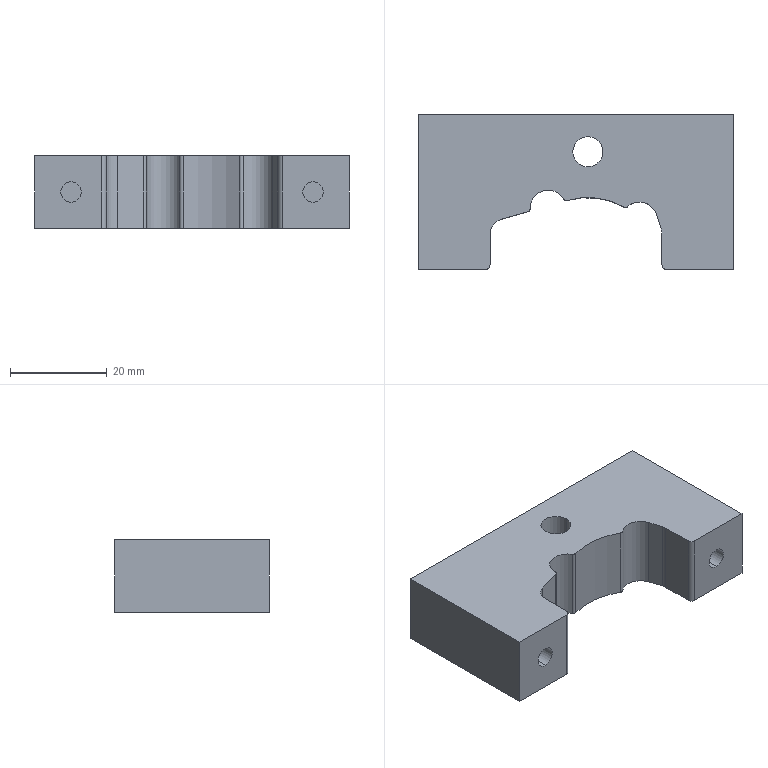NC program | Mastercam | posted with a generic post
Lines 25 to 726 of 2481:
N230 T9 M6
N240 G0 G90 G17 G54 X-45.614 Y-30.265 A0. S6000 M3
N250 G43 H9 Z50.
N260 Z2.
N270 G1 Z-15.75 F2000.
N280 X-45.889 Y-29.487 Z-15.877 F4000.
N290 G3 X-46.313 Y-28.813 Z-16. I-1.697 J-.599
N300 G2 X-47.51 Y-26.707 I5.557 J4.549
N310 X-47.895 Y-24.67 I7.524 J2.477
N320 X-47.955 Y-22.296 I47.214 J2.374
N330 X-47.943 Y-21.288 I47.274 J0.
N340 X-47.932 Y-20.029 I986.819 J-8.394
N350 G1 X-47.929 Y-19.714
N360 X-47.612 Y11.998
N370 X-47.499 Y22.913
N380 G2 X-47.09 Y25.288 I7.557 J-.078
N390 X-44.537 Y28.308 I5.258 J-1.857
N400 X-41.791 Y29.334 I4.597 J-8.114
N410 X-38.089 Y29.777 I4.617 J-22.923
N420 X-32.309 Y29.894 I5.78 J-143.246
N430 X-31.772 Y29.892 I0. J-143.363
N440 X-29.817 Y29.897 I3.277 J-998.552
N450 G1 X-29.492
N460 X2.98 Y29.9
N470 X35.449
N480 G2 X36.585 Y29.901 I1.136 J-880.668
N490 X40.411 Y29.892 I0. J-880.669
N500 X43.057 Y29.37 I-.083 J-7.387
N510 X45.814 Y26.904 I-2.177 J-5.207
N520 X46.836 Y24.158 I-8.139 J-4.595
N530 X47.277 Y20.458 I-22.99 J-4.615
N540 X47.393 Y14.679 I-143.703 J-5.779
N550 X47.392 Y14.141 I-143.819 J0.
N560 X47.396 Y12.512 I-914.774 J-3.05
N570 G1 X47.397 Y12.187
N580 X47.4 Y-20.286
N590 G2 X47.401 Y-20.936 I-181.849 J-.65
N600 X47.39 Y-22.995 I-181.85 J0.
N610 X46.829 Y-25.653 I-7.232 J.136
N620 X44.318 Y-28.363 I-5.202 J2.303
N630 X41.384 Y-29.394 I-4.683 J8.636
N640 X37.72 Y-29.789 I-4.561 J25.118
N650 X31.559 Y-29.897 I-6.161 J176.47
N660 X30.765 Y-29.895 I0. J176.578
N670 G1 X30.439
N680 X-2.036 Y-29.9
N690 X-34.504
N700 X-40.449 Y-29.891
N710 G2 X-42.643 Y-29.509 I.097 J7.049
N720 X-45.36 Y-27.368 I1.999 J5.331
N730 X-46.578 Y-24.594 I7.011 J4.733
N740 X-47.068 Y-21.166 I18.144 J4.342
N750 X-47.178 Y-16.743 I88.951 J4.423
N760 X-47.173 Y-15.771 I89.061 J0.
N770 X-47.13 Y-9.905 I968.214 J-4.162
N780 G1 X-47.127 Y-9.581
N790 X-46.811 Y21.335
N800 G2 X-46.545 Y23.383 I8.429 J-.053
N810 X-44.207 Y26.771 I6.177 J-1.762
N820 X-41.382 Y28.209 I5.544 J-7.399
N830 X-37.947 Y28.896 I5.105 J-16.599
N840 X-32.805 Y29.157 I5.493 J-57.43
N850 X-23.221 Y29.203 I9.584 J-998.899
N860 X-20.74 Y29.2 I0. J-998.945
N870 G1 X-20.415
N880 X12.054
N890 X38.75 Y29.191
N900 X38.76
N910 G2 X40.794 Y28.949 I0. J-8.644
N920 X44.217 Y26.656 I-1.659 J-6.178
N930 X45.685 Y23.834 I-7.243 J-5.561
N940 X46.388 Y20.391 I-16.3 J-5.124
N950 X46.65 Y15.576 I-54.549 J-5.373
N960 X46.704 Y5.699 I-910.196 J-9.877
N970 X46.7 Y3.178 I-910.25 J0.
N980 G1 Y2.853
N990 X46.691 Y-21.246
N1000 Y-21.257
N1010 G2 X46.451 Y-23.287 I-8.672 J0.
N1020 X44.161 Y-26.713 I-6.178 J1.651
N1030 X41.339 Y-28.183 I-5.562 J7.231
N1040 X37.896 Y-28.888 I-5.124 J16.276
N1050 X33.08 Y-29.149 I-5.375 J54.481
N1060 X23.203 Y-29.203 I-9.877 J908.925
N1070 X20.681 Y-29.2 I0. J908.979
N1080 G1 X20.357
N1090 X-12.112
N1100 X-38.82 Y-29.19
N1110 X-38.83
N1120 G2 X-41.221 Y-28.777 I0. J7.137
N1130 X-44.103 Y-26.61 I2.341 J6.114
N1140 X-45.546 Y-23.777 I7.31 J5.507
N1150 X-46.22 Y-20.326 I16.303 J4.976
N1160 X-46.436 Y-15.507 I54.432 J4.852
N1170 G1 Y-14.598
N1180 G2 X-46.363 Y-3.108 I897.862 J0.
N1190 G1 X-46.36 Y-2.783
N1200 X-46.129 Y19.67
N1210 G2 X-45.821 Y22.09 I9.687 J-.004
N1220 X-43.504 Y25.623 I6.853 J-1.968
N1230 X-40.379 Y27.338 I6.19 J-7.578
N1240 X-36.6 Y28.145 I5.691 J-17.4
N1250 X-31.451 Y28.441 I5.758 J-55.184
N1260 X-21.727 Y28.503 I9.724 J-760.399
N1270 X-19.373 Y28.499 I0. J-760.461
N1280 G1 X-19.048
N1290 X13.422 Y28.5
N1300 X37.185 Y28.492
N1310 X37.233
N1320 G2 X39.63 Y28.181 I0. J-9.402
N1330 X43.151 Y25.845 I-2. J-6.838
N1340 X44.851 Y22.717 I-7.645 J-6.179
N1350 X45.649 Y18.941 I-17.546 J-5.681
N1360 X45.942 Y13.795 I-55.737 J-5.753
N1370 X46.003 Y4.073 I-769.313 J-9.722
N1380 X45.999 Y1.717 I-769.374 J0.
N1390 G1 Y1.392
N1400 X45.989 Y-19.784
N1410 Y-19.791
N1420 G2 X45.642 Y-22.262 I-8.962 J0.
N1430 X43.244 Y-25.734 I-6.83 J2.153
N1440 X40.109 Y-27.387 I-6.151 J7.865
N1450 X36.343 Y-28.16 I-5.655 J17.992
N1460 X31.204 Y-28.443 I-5.741 J57.339
N1470 X21.208 Y-28.502 I-9.996 J840.155
N1480 X18.804 Y-28.499 I0. J840.214
N1490 G1 X18.479 Y-28.5
N1500 X-13.99
N1510 X-37.099 Y-28.493
N1520 X-37.145
N1530 G2 X-39.581 Y-28.156 I0. J8.963
N1540 X-43.064 Y-25.764 I2.114 J6.813
N1550 X-44.718 Y-22.618 I7.782 J6.097
N1560 X-45.471 Y-18.838 I17.743 J5.502
N1570 X-45.711 Y-13.691 I56.177 J5.193
N1580 X-45.714 Y-11.688 I772.695 J2.003
N1590 X-45.648 Y-1.614 I772.698 J0.
N1600 G1 X-45.644 Y-1.289
N1610 X-45.442 Y18.245
N1620 G2 X-45.128 Y20.796 I11.216 J-.086
N1630 X-42.518 Y24.805 I7.408 J-1.969
N1640 X-39.448 Y26.501 I6.467 J-8.078
N1650 X-35.684 Y27.368 I5.973 J-17.338
N1660 X-30.512 Y27.719 I6.026 J-50.413
N1670 X-21.626 Y27.8 I8.886 J-485.482
N1680 X-20.04 Y27.798 I0. J-485.563
N1690 G1 X-19.715
N1700 X12.755 Y27.8
N1710 X35.887 Y27.787
N1720 G2 X38.491 Y27.435 I-.066 J-10.297
N1730 X42.438 Y24.72 I-2.176 J-7.39
N1740 X44.193 Y21.249 I-8.694 J-6.574
N1750 X44.972 Y17.172 I-20.126 J-5.957
N1760 X45.246 Y11.73 I-67.431 J-6.124
N1770 X45.304 Y1.065 I-987.723 J-10.665
N1780 X45.3 Y-1.639 I-987.781 J0.
N1790 G1 Y-1.964
N1800 X45.29 Y-18.262
N1810 G2 X44.979 Y-20.833 I-10.873 J.011
N1820 X42.343 Y-24.84 I-7.391 J1.991
N1830 X39.269 Y-26.519 I-6.448 J8.154
N1840 X35.509 Y-27.374 I-5.959 J17.514
N1850 X30.34 Y-27.721 I-6.019 J51.043
N1860 X21.457 Y-27.801 I-8.883 J492.934
N1870 X19.87 Y-27.798 I0. J493.014
N1880 G1 X19.545
N1890 X-12.926 Y-27.8
N1900 X-35.728 Y-27.789
N1910 G2 X-38.335 Y-27.439 I.05 J10.265
N1920 X-42.147 Y-24.884 I2.152 J7.333
N1930 X-43.834 Y-21.799 I8.025 J6.392
N1940 X-44.674 Y-18.024 I17.221 J5.811
N1950 X-44.979 Y-12.845 I49.968 J5.537
N1960 X-44.997 Y-8.745 I478.968 J4.1
N1970 X-44.954 Y-2.372 I478.986 J0.
N1980 G1 X-44.951 Y-2.047
N1990 X-44.755 Y16.84
N2000 G2 X-44.504 Y19.282 I13.738 J-.174
N2010 X-41.214 Y24.29 I8.022 J-1.687
N2020 X-37.776 Y25.953 I6.71 J-9.482
N2030 X-33.725 Y26.736 I6.138 J-20.895
N2040 X-27.946 Y27.041 I6.433 J-67.056
N2050 X-17.339 Y27.103 I10.607 J-910.669
N2060 X-14.9 Y27.099 I0. J-910.731
N2070 G1 X-14.575
N2080 X17.894 Y27.1
N2090 X34.174 Y27.092
N2100 X34.184
N2110 G2 X36.588 Y26.893 I0. J-14.562
N2120 X41.682 Y23.722 I-1.447 J-8.003
N2130 X43.407 Y20.291 I-9.216 J-6.782
N2140 X44.221 Y16.227 I-20.23 J-6.168
N2150 X44.531 Y10.771 I-63.111 J-6.321
N2160 X44.602 Y.838 I-696.262 J-9.933
N2170 X44.599 Y-1.31 I-696.333 J0.
N2180 G1 Y-1.635
N2190 X44.587 Y-16.97
N2200 G2 X44.315 Y-19.461 I-12.601 J.113
N2210 X41.285 Y-24.134 I-7.919 J1.816
N2220 X37.858 Y-25.885 I-6.8 J9.079
N2230 X33.789 Y-26.715 I-6.184 J19.95
N2240 X28.328 Y-27.03 I-6.329 J62.114
N2250 X18.54 Y-27.102 I-9.788 J669.314
N2260 X16.571 Y-27.099 I0. J669.386
N2270 G1 X16.246
N2280 X-16.223 Y-27.1
N2290 X-34.135 Y-27.091
N2300 G2 X-36.581 Y-26.866 I.023 J13.644
N2310 X-41.338 Y-23.95 I1.566 J7.893
N2320 X-43.148 Y-20.518 I8.686 J6.774
N2330 X-43.986 Y-16.424 I19.104 J6.044
N2340 X-44.267 Y-10.947 I58.989 J5.766
N2350 X-44.278 Y-7.384 I596.981 J3.563
N2360 X-44.226 Y.49 I596.992 J0.
N2370 G1 X-44.223 Y.815
N2380 X-44.067 Y15.479
N2390 G2 X-43.781 Y18.264 I15.659 J-.203
N2400 X-40.26 Y23.544 I8.409 J-1.794
N2410 X-36.853 Y25.184 I6.889 J-9.948
N2420 X-32.459 Y26.032 I6.53 J-22.026
N2430 X-26.692 Y26.336 I6.554 J-69.681
N2440 X-15.997 Y26.403 I10.695 J-855.879
N2450 X-13.643 Y26.399 I0. J-855.946
N2460 G1 X-13.318
N2470 X19.151 Y26.4
N2480 X32.834 Y26.391
N2490 G2 X35.599 Y26.155 I-.008 J-16.392
N2500 X40.957 Y22.737 I-1.575 J-8.378
N2510 X42.646 Y19.334 I-9.716 J-6.944
N2520 X43.481 Y15.285 I-20.512 J-6.338
N2530 X43.818 Y9.82 I-60.646 J-6.486
N2540 X43.9 Y.335 I-548.288 J-9.485
N2550 X43.898 Y-1.295 I-548.37 J0.
N2560 G1 Y-1.62
N2570 X43.892 Y-15.303
N2580 Y-15.311
N2590 G2 X43.663 Y-18.059 I-16.613 J0.
N2600 X40.27 Y-23.433 I-8.379 J1.532
N2610 X36.869 Y-25.135 I-6.954 J9.645
N2620 X32.817 Y-25.977 I-6.346 J20.37
N2630 X27.351 Y-26.317 I-6.49 J60.165
N2640 X17.864 Y-26.4 I-9.487 J543.312
N2650 X16.235 Y-26.398 I0. J543.395
N2660 G1 X15.91
N2670 X-16.561 Y-26.4
N2680 X-32.853 Y-26.389
N2690 G2 X-35.664 Y-26.111 I.061 J14.961
N2700 X-40.665 Y-22.896 I1.77 J8.248
N2710 X-42.403 Y-19.486 I9.334 J6.908
N2720 X-43.243 Y-15.413 I19.709 J6.188
N2730 X-43.545 Y-9.932 I58.101 J5.944
N2740 X-43.564 Y-5.625 I492.643 J4.307
N2750 X-43.521 Y.862 I492.662 J0.
N2760 G1 X-43.518 Y1.187
N2770 X-43.378 Y14.231
N2780 G2 X-43.132 Y16.942 I18.18 J-.284
N2790 X-39.225 Y22.882 I8.819 J-1.545
N2800 X-35.461 Y24.574 I7.187 J-10.954
N2810 X-31.112 Y25.345 I6.578 J-24.472
N2820 X-25.031 Y25.64 I6.879 J-78.864
N2830 X-14.126 Y25.702 I10.905 J-956.982
N2840 X-11.664 Y25.699 I0. J-957.044
N2850 G1 X-11.339
N2860 X21.13 Y25.7
N2870 X31.567 Y25.69
N2880 G2 X34.256 Y25.494 I-.058 J-19.277
N2890 X40.287 Y21.715 I-1.302 J-8.781
N2900 X42.035 Y17.954 I-10.584 J-7.206
N2910 X42.833 Y13.594 I-23.775 J-6.601
N2920 X43.138 Y7.507 I-76.485 J-6.888
N2930 X43.202 Y-3.674 I-972.393 J-11.181
N2940 X43.199 Y-6.187 I-972.457 J0.
N2950 G1 Y-6.512
N2960 G2 X43.201 Y-8.586 I-990.829 J-2.074
N2970 X43.185 Y-14.374 I-990.831 J0.
N2980 X42.926 Y-17.13 I-16.565 J.166
N2990 X39.259 Y-22.756 I-8.703 J1.664
N3000 X35.5 Y-24.522 I-7.226 J10.499
N3010 X31.137 Y-25.328 I-6.61 J23.555
N3020 X25.048 Y-25.637 I-6.893 J75.679
N3030 X13.866 Y-25.702 I-11.182 J960.7
N3040 X11.353 Y-25.699 I0. J960.765
N3050 G1 X11.028
N3060 X-21.441 Y-25.7
N3070 X-31.562 Y-25.688
N3080 G2 X-34.288 Y-25.462 I.1 J17.724
N3090 X-39.982 Y-21.887 I1.465 J8.657
N3100 X-41.782 Y-18.117 I10.155 J7.164
N3110 X-42.581 Y-13.733 I22.793 J6.417
N3120 X-42.843 Y-7.631 I72.86 J6.183
N3130 X-42.846 Y-5.471 I876.429 J2.16
N3140 X-42.774 Y5.742 I876.432 J0.
N3150 G1 X-42.771 Y6.066
N3160 G2 X-42.681 Y13.282 I705.047 J-5.15
N3170 X-42.33 Y16.407 I16.546 J-.274
N3180 X-38.628 Y21.941 I8.971 J-1.996
N3190 X-34.898 Y23.732 I7.395 J-10.62
N3200 X-30.536 Y24.583 I6.779 J-23.139
N3210 X-24.432 Y24.925 I7.042 J-71.036
N3220 X-13.845 Y25.001 I10.587 J-735.463
N3230 X-11.704 Y24.999 I0. J-735.539
N3240 G1 X-11.379
N3250 X21.091 Y25.
N3260 X30.566 Y24.986
N3270 G2 X33.661 Y24.706 I-.041 J-17.712
N3280 X39.562 Y20.801 I-1.714 J-9.003
N3290 X41.29 Y17.061 I-10.97 J-7.335
N3300 X42.104 Y12.71 I-23.95 J-6.732
N3310 X42.429 Y6.617 I-74.089 J-7.016
N3320 X42.501 Y-4.23 I-811.991 J-10.847
N3330 X42.499 Y-6.433 I-812.063 J0.
N3340 G1 Y-6.758
N3350 G2 X42.502 Y-8.488 I-526.727 J-1.73
N3360 X42.479 Y-13.332 I-526.73 J0.
N3370 X42.136 Y-16.485 I-15.85 J.133
N3380 X38.389 Y-22.001 I-8.915 J2.024
N3390 X34.652 Y-23.762 I-7.36 J10.771
N3400 X30.295 Y-24.594 I-6.751 J23.53
N3410 X24.197 Y-24.928 I-7.026 J72.615
N3420 X13.615 Y-25.002 I-10.582 J756.421
N3430 X11.47 Y-24.999 I0. J756.495
N3440 G1 X11.145
N3450 X-21.325 Y-25.
N3460 X-30.479 Y-24.985
N3470 G2 X-33.594 Y-24.687 I.054 J17.024
N3480 X-39.196 Y-21.051 I1.778 J8.874
N3490 X-41.004 Y-17.304 I10.349 J7.301
N3500 X-41.835 Y-12.924 I22.641 J6.564
N3510 X-42.119 Y-7.143 I66.163 J6.156
N3520 X-42.133 Y-3.086 I599.653 J4.057
N3530 X-42.084 Y4.619 I599.667 J0.
N3540 G1 X-42.08 Y4.944
N3550 G2 X-41.99 Y12.161 I621.71 J-4.194
N3560 X-41.673 Y15.233 I18.347 J-.343
N3570 X-37.509 Y21.381 I9.315 J-1.824
N3580 X-33.786 Y23.065 I7.439 J-11.487
N3590 X-29.097 Y23.918 I6.968 J-24.988
N3600 X-22.691 Y24.235 I7.213 J-80.934
N3610 X-11.23 Y24.302 I11.461 J-975.753
N3620 X-8.673 Y24.299 I0. J-975.82
N3630 G1 X-8.348
N3640 X24.122 Y24.3
N3650 G2 X25.391 Y24.302 I1.269 J-380.369
N3660 X29.721 Y24.277 I0. J-380.371
N3670 X32.818 Y23.968 I-.185 J-17.515
N3680 X38.703 Y20.109 I-1.828 J-9.204
N3690 X40.486 Y16.395 I-10.852 J-7.497
N3700 X41.355 Y12.039 I-23.201 J-6.892
N3710 X41.716 Y5.929 I-69.104 J-7.154
N3720 X41.8 Y-4.332 I-627.054 J-10.261
N3730 X41.798 Y-6.155 I-627.138 J0.
N3740 G1 Y-6.48
N3750 G2 X41.802 Y-8.038 I-314.958 J-1.558
N3760 X41.771 Y-12.422 I-314.962 J0.
N3770 X41.415 Y-15.559 I-16.236 J.257
N3780 X37.761 Y-21.093 I-9.121 J2.049
N3790 X34.056 Y-22.935 I-7.54 J10.515
N3800 X29.691 Y-23.837 I-6.926 J22.506
N3810 X23.904 Y-24.204 I-6.946 J63.669
N3820 X14.024 Y-24.299 I-9.88 J514.383
N3830 X12.46 Y-24.297 I0. J514.478
N3840 G1 X12.135
N3850 X-20.336 Y-24.3
N3860 X-29.155 Y-24.287
N3870 G2 X-32.176 Y-24.059 I.047 J20.752
N3880 X-36.303 Y-22.371 I1.452 J9.444
N3890 X-39.176 Y-19.029 I5.927 J8.002
N3900 X-40.651 Y-14.907 I13.556 J7.173
N3910 X-41.272 Y-9.945 I32.534 J6.594
N3920 X-41.429 Y-3.57 I129.288 J6.375
N3930 X-41.426 Y-2.62 I129.445 J0.
N3940 X-41.377 Y5.199 I994.994 J-2.291
N3950 G1 X-41.374 Y5.524
N3960 G2 X-41.283 Y11.474 I270.041 J-1.139
N3970 X-40.908 Y14.575 I17.298 J-.518
N3980 X-36.68 Y20.637 I9.481 J-2.108
N3990 X-32.973 Y22.318 I7.546 J-11.708
N4000 X-28.289 Y23.191 I7.08 J-24.98
N4010 X-21.876 Y23.527 I7.321 J-78.423
N4020 X-10.755 Y23.601 I11.121 J-831.422
N4030 X-8.503 Y23.599 I0. J-831.496
N4040 G1 X-8.178
N4050 X24.292 Y23.6
N4060 G2 X25.319 Y23.603 I1.027 J-156.116
N4070 X29.299 Y23.553 I0. J-156.119
N4080 X32.47 Y23.118 I-.468 J-15.204
N4090 X37.894 Y19.365 I-2.404 J-9.27
N4100 X39.707 Y15.674 I-10.863 J-7.626
N4110 X40.615 Y11.317 I-22.815 J-7.025
N4120 X41.005 Y5.196 I-65.895 J-7.274
N4130 X41.099 Y-5.006 I-551.649 J-10.202
N4140 X41.097 Y-6.57 I-551.743 J0.
N4150 G1 Y-6.895
N4160 G2 X41.101 Y-7.996 I-162.501 J-1.101
N4170 X41.062 Y-11.556 I-162.505 J0.
N4180 X40.689 Y-14.684 I-16.474 J.377
N4190 X36.75 Y-20.476 I-9.363 J2.133
N4200 X33.052 Y-22.246 I-7.596 J11.121
N4210 X28.352 Y-23.169 I-7.12 J23.832
N4220 X22.257 Y-23.516 I-7.219 J73.081
N4230 X11.67 Y-23.601 I-10.587 J663.08
N4240 X9.849 Y-23.598 I0. J663.165
N4250 G1 X9.525
N4260 X-22.946 Y-23.6
N4270 G2 X-24.197 Y-23.602 I-1.251 J336.019
N4280 X-28.55 Y-23.574 I0. J336.021
N4290 X-31.622 Y-23.275 I.246 J18.462
N4300 X-37.812 Y-19.193 I1.742 J9.373
N4310 X-39.541 Y-15.473 I11.187 J7.465
N4320 X-40.412 Y-10.765 I23.978 J6.868
N4330 X-40.695 Y-4.669 I73.642 J6.476
N4340 X-40.706 Y-.985 I603. J3.684
N4350 X-40.605 Y10.089 I603.011 J0.
N4360 X-40.323 Y13.094 I21.279 J-.481
N4370 X-38.701 Y17.151 I10.151 J-1.707
N4380 X-35.134 Y20.34 I8.494 J-5.91
N4390 X-31.059 Y21.875 I7.545 J-13.855
N4400 X-26.103 Y22.595 I7.162 J-31.88
N4410 X-19.092 Y22.853 I7.641 J-111.963
N4420 X-9.723 Y22.898 I9.369 J-980.312
N4430 G1 X-8.664 Y22.897
N4440 X-8.34 Y22.898
N4450 X24.132 Y22.9
N4460 G2 X24.879 Y22.903 I.747 J-103.905
N4470 X28.511 Y22.839 I0. J-103.908
N4480 X31.679 Y22.376 I-.596 J-15.166
N4490 X37.082 Y18.644 I-2.518 J-9.423
N4500 X38.928 Y14.973 I-10.786 J-7.723
N4510 X39.874 Y10.617 I-22.418 J-7.148
N4520 X40.283 Y4.818 I-60.555 J-7.182
N4530 X40.396 Y-4.825 I-409.971 J-9.643
N4540 X40.394 Y-5.989 I-410.084 J0.
N4550 G1 X40.395 Y-6.314
N4560 G2 X40.4 Y-7.353 I-106.992 J-1.039
N4570 X40.337 Y-11.024 I-106.997 J0.
N4580 X39.872 Y-14.192 I-15.098 J.596
N4590 X36.132 Y-19.591 I-9.423 J2.533
N4600 X32.46 Y-21.433 I-7.747 J10.866
N4610 X27.753 Y-22.419 I-7.265 J22.935
N4620 X21.642 Y-22.802 I-7.344 J68.221
N4630 X11.373 Y-22.898 I-10.269 J547.19
N4640 X9.875 Y-22.897 I0. J547.286
N4650 G1 X9.55
N4660 X-22.921 Y-22.9
N4670 G2 X-23.925 Y-22.903 I-1.004 J182.05
N4680 X-27.908 Y-22.859 I0. J182.053
N4690 X-31.012 Y-22.499 I.43 J17.255
N4700 X-37.101 Y-18.317 I2.053 J9.514
N4710 X-38.808 Y-14.609 I11.499 J7.54
N4720 X-39.684 Y-9.909 I24.253 J6.953
N4730 X-39.979 Y-3.811 I72.693 J6.577
N4740 X-39.997 Y.176 I438.19 J3.987
N4750 X-39.902 Y9.345 I438.208 J0.
N4760 X-39.504 Y12.772 I19.626 J-.542
N4770 X-35.328 Y18.978 I9.827 J-2.104
N4780 G3 X-35.252 Y19.039 I-.461 J.654
N4790 G2 X-34.091 Y19.801 I3.212 J-3.631
N4800 X-29.698 Y21.281 I7.916 J-16.231
N4810 X-24.447 Y21.941 I7.306 J-36.914
N4820 X-16.812 Y22.166 I8.04 J-143.274
N4830 X-9.319 Y22.196 I7.62 J-966.616
N4840 G1 X-8.994
N4850 X23.481 Y22.199
N4860 G2 X24.146 Y22.202 I.665 J-80.375
N4870 X27.9 Y22.114 I0. J-80.378
N4880 X31.083 Y21.584 I-.782 J-14.51
N4890 X36.395 Y17.768 I-2.824 J-9.535
N4900 X38.33 Y13.733 I-11.322 J-7.912
N4910 X39.242 Y9.056 I-24.823 J-7.268
N4920 X39.612 Y2.631 I-74.522 J-7.516
N4930 X39.687 Y-5.093 I-399.679 J-7.724
N4940 X39.666 Y-9.215 I-399.754 J0.
N4950 X39.323 Y-12.632 I-20.086 J.289
N4960 X35.741 Y-18.535 I-9.779 J1.895
N4970 G3 X35.641 Y-18.636 I.512 J-.615
N4980 G2 X34.013 Y-19.831 I-3.4 J2.922
N4990 X29.297 Y-21.342 I-8.227 J17.569
N5000 X24.069 Y-21.957 I-7.304 J39.56
N5010 X16.117 Y-22.171 I-8.264 J159.146
N5020 X9.928 Y-22.195 I-6.868 J965.426
N5030 G1 X9.603
N5040 X-22.872 Y-22.2
N5050 G2 X-23.584 Y-22.202 I-.712 J113.082
N5060 X-27.237 Y-22.143 I0. J113.084
N5070 X-30.361 Y-21.731 I.582 J16.476
N5080 X-34.697 Y-19.462 I2.324 J9.716
N5090 X-36.045 Y-18.103 I2.436 J3.765
N5100 X-38.105 Y-13.729 I11.845 J8.25
N5110 X-38.962 Y-9.052 I25.355 J7.067
N5120 X-39.27 Y-2.624 I74.554 J6.784
N5130 X-39.289 Y.988 I345.437 J3.612
N5140 X-39.212 Y8.247 I345.456 J0.
N5150 X-38.861 Y11.624 I21.629 J-.544
N5160 X-36.714 Y16.254 I10.249 J-1.939
N5170 G3 X-36.552 Y16.627 I-.628 J.495
N5180 G2 X-32.791 Y20.09 I4.052 J-.627
N5190 G3 X-30.119 Y20.513 I-5.79 J45.179
N5200 G2 X-21.658 Y21.342 I10.232 J-60.821
N5210 X-12.109 Y21.49 I9.549 J-308.731
N5220 X-11.484 Y21.489 I0. J-308.879
N5230 G1 X-11.159 Y21.49
N5240 X21.319 Y21.5
N5250 G2 X22.221 Y21.503 I.902 J-148.467
N5260 X26.322 Y21.446 I0. J-148.47
N5270 X29.803 Y20.989 I-.537 J-17.567
N5280 X31.963 Y20.184 I-2.565 J-10.192
N5290 G3 X32.389 Y20.094 I.426 J.961
N5300 X32.5 Y20.1 I0. J1.051
N5310 G2 X36.425 Y17.186 I0. J-4.1
N5320 G3 X37.132 Y15.074 I92.359 J29.739
N5330 G2 X38.56 Y8.104 I-30.635 J-9.91
N5340 X38.917 Y1.377 I-86.052 J-7.939
N5350 X38.98 Y-4.864 I-309.43 J-6.241
N5360 X38.962 Y-8.185 I-309.493 J0.
N5370 X38.65 Y-11.566 I-21.707 J.298
N5380 X36.729 Y-15.998 I-10.316 J1.839
N5390 G3 X36.581 Y-16.39 I.649 J-.468
N5400 G2 X35.558 Y-18.731 I-4.081 J.39
N5410 G3 X35.173 Y-19.427 Z-15.92 I1.343 J-1.199
N5420 G1 X34.971 Y-20.12 Z-15.848
N5430 G3 X34.936 Y-20.369 Z-15.823 I.859 J-.249
N5440 X35.222 Y-21.025 Z-15.75 I.894 J0.
N5450 X35.455 Y-21.181 I.608 J.656 F9500.
N5460 G1 X37.248 Y-22.007
N5470 G3 X37.623 Y-22.09 I.375 J.811
N5480 X38.5 Y-21.368 I0. J.894
N5490 X40.56 Y-.212 I-107.608 J21.156
N5500 X40.436 Y4.998 I-109.668 J0.
N5510 G1 X39.73 Y19.83
N5520 G3 X37.942 Y21.535 I-1.788 J-.085
N5530 X36.194 Y20.131 I0. J-1.79
N5540 X36.153 Y19.806 Z-15.783 I1.748 J-.386 F4000.
N5550 G1 X36.131 Y19.145 Z-15.848
N5560 X36.107 Y18.424 Z-15.92
N5570 G3 X36.106 Y18.364 Z-15.926 I1.799 J-.06
N5580 X36.257 Y17.643 Z-16. I1.8 J0.
N5590 G2 X36.6 Y16. I-3.757 J-1.643
N5600 G3 X36.904 Y13.882 I16.525 J1.29
N5610 X37.023 Y13.251 I268.844 J50.29
N5620 G2 X38.112 Y3.8 I-58.66 J-11.546
N5630 X38.27 Y-4.47 I-215.959 J-8.27
N5640 X38.249 Y-7.466 I-216.117 J0.
N5650 X37.908 Y-10.863 I-20.941 J.384
N5660 X36.878 Y-13.893 I-12.715 J2.634
N5670 G3 X36.664 Y-14.386 I22.91 J-10.224
N5680 X36.6 Y-14.7 I.736 J-.314
N5690 G1 Y-15.025
N5700 G2 X36.607 Y-15.509 I-16.707 J-.484
N5710 X36.587 Y-16.324 I-16.714 J0.
N5720 X36.549 Y-16.647 I-4.087 J.324
N5730 G3 X36.526 Y-16.931 Z-15.972 I1.777 J-.284
N5740 X37.738 Y-18.632 Z-15.75 I1.8 J0.
N5750 X38.326 Y-18.731 I.588 J1.701 F9500.
N5760 X40.126 Y-16.932 I0. J1.8
N5770 G1 X40.158 Y16.697
N5780 Y16.699
N5790 G3 X38.358 Y18.499 I-1.8 J0.
N5800 X37.838 Y18.422 I0. J-1.8
N5810 X36.558 Y16.699 Z-15.979 I.52 J-1.723 F4000.
N5820 X36.571 Y16.486 Z-16. I1.8 J0.
N5830 G2 X36.605 Y15.673 I-9.62 J-.813
N5840 X36.6 Y15.351 I-9.654 J0.
N5850 G1 Y15.026
N5860 G3 X36.594 Y14.38 I34.765 J-.646
N5870 X36.631 Y12.766 I34.771 J0.
N5880 X37.001 Y9.001 I109.728 J8.873
N5890 G2 X37.522 Y-.647 I-111.822 J-10.879
N5900 X37.56 Y-3.998 I-147.874 J-3.351
N5910 X37.537 Y-6.643 I-147.912 J0.
N5920 X37.195 Y-10.031 I-21.117 J.422
N5930 X36.636 Y-12.118 I-18.917 J3.939
N5940 G3 X36.591 Y-12.51 I1.678 J-.392
N5950 X36.6 Y-12.682 I1.723 J0.
N5960 G1 Y-13.006
N5970 Y-15.279
N5980 G3 X38.087 Y-17.052 Z-15.75 I1.8 J0.
N5990 X38.4 Y-17.079 I.313 J1.773 F9500.
N6000 X40.2 Y-15.279 I0. J1.8
N6010 G1 Y14.047
N6020 G3 X38.4 Y15.847 I-1.8 J0.
N6030 X38.087 Y15.819 I0. J-1.8
N6040 X36.6 Y14.047 Z-16. I.313 J-1.772 F4000.
N6050 G1 Y13.56
N6060 X36.612 Y6.477
N6070 G2 X36.837 Y-2.318 I-424.904 J-15.296
N6080 X36.85 Y-3.639 I-69.63 J-1.321
N6090 X36.78 Y-6.756 I-69.643 J0.
N6100 X36.6 Y-8.6 I-28.132 J1.819
N6110 G1 Y-8.925
N6120 Y-12.821
N6130 G3 X38.087 Y-14.594 Z-15.75 I1.8 J0.
N6140 X38.4 Y-14.621 I.313 J1.773 F9500.
N6150 X40.2 Y-12.821 I0. J1.8
N6160 G1 Y7.877
N6170 G3 X38.4 Y9.677 I-1.8 J0.
N6180 X38.087 Y9.65 I0. J-1.8
N6190 X36.6 Y7.877 Z-16. I.313 J-1.773 F4000.
N6200 G1 Y7.39
N6210 Y-9.169
N6220 G3 X36.776 Y-9.945 Z-15.92 I1.8 J0.
N6230 G1 X37.304 Y-11.049 Z-15.798
N6240 G2 X37.452 Y-11.511 Z-15.75 I-1.624 J-.777
N6250 X37.477 Y-11.726 I-1.772 J-.315 F9500.
N6260 G1 X37.778 Y-17.133
N6270 G2 X37.781 Y-17.233 I-1.797 J-.1
N6280 X37.133 Y-18.616 I-1.8 J0.
N6290 X36.241 Y-19.014 Z-15.848 I-1.152 J1.383 F4000.
N6300 G1 X35.527 Y-19.118 Z-15.92
N6310 G3 X34.784 Y-19.405 Z-16. I.26 J-1.782
N6320 G2 X32.576 Y-20.111 I-2.353 J3.552
N6330 G3 X29.861 Y-20.541 I7.68 J-57.234
N6340 G2 X21.405 Y-21.347 I-10.2 J62.292
N6350 X11.859 Y-21.49 I-9.546 J318.035
N6360 G1 X11.235
N6370 X10.909
N6380 X-21.569 Y-21.5
N6390 G2 X-22.41 Y-21.503 I-.841 J120.724
N6400 X-26.257 Y-21.441 I0. J120.727
N6410 X-29.351 Y-21.054 I.615 J17.457
N6420 X-31.787 Y-20.177 I2.421 J10.554
N6430 G3 X-32.13 Y-20.1 I-.343 J-.723
N6440 G1 X-32.455
N6450 X-32.487
N6460 G2 X-36.557 Y-16.665 I0. J4.128
N6470 G3 X-37.235 Y-14.194 I-94.013 J-24.466
N6480 G2 X-38.346 Y-7.251 I36.182 J9.352
N6490 X-38.575 Y-.147 I110.259 J7.104
N6500 X-38.574 Y.099 I110.488 J0.
N6510 X-38.58 Y1.785 I231.551 J1.686
N6520 X-38.513 Y7.374 I231.557 J0.
N6530 X-38.163 Y10.743 I22.1 J-.596
N6540 X-36.938 Y14.155 I12.105 J-2.419
N6550 G3 X-36.672 Y14.715 I-21.126 J10.372
N6560 X-36.6 Y15.047 I-.728 J.332
N6570 G1 Y15.372
N6580 G2 X-36.609 Y15.73 I6.966 J.358
N6590 X-36.549 Y16.647 I6.975 J0.
N6600 G3 X-36.526 Y16.931 Z-15.972 I-1.777 J.284
N6610 X-37.738 Y18.632 Z-15.75 I-1.8 J0.
N6620 X-38.326 Y18.731 I-.588 J-1.701 F9500.
N6630 X-40.126 Y16.931 I0. J-1.8
N6640 G1 Y16.917
N6650 X-39.856 Y-17.999
N6660 G3 X-38.056 Y-19.785 I1.8 J.014
N6670 X-37.165 Y-19.549 I0. J1.8
N6680 X-36.256 Y-17.985 Z-15.939 I-.891 J1.564 F4000.
N6690 X-36.361 Y-17.379 Z-16. I-1.8 J0.
N6700 G2 X-36.606 Y-15.912 I4.264 J1.467
N6710 X-36.6 Y-15.675 I4.509 J0.
N6720 G3 X-36.815 Y-13.568 I-15.546 J-.52
N6730 X-37.009 Y-12.295 I-398.545 J-60.095
N6740 G2 X-37.811 Y-2.863 I68.232 J10.553
N6750 X-37.867 Y1.757 I191.316 J4.62
N6760 X-37.801 Y6.768 I191.372 J0.
N6770 X-37.404 Y10.163 I20.634 J-.694
N6780 X-36.644 Y12.674 I20.299 J-4.77
N6790 G3 X-36.6 Y12.936 I-.756 J.262
N6800 G1 Y13.261
N6810 Y15.534
N6820 G3 X-38.087 Y17.306 Z-15.75 I-1.8 J0.
N6830 X-38.4 Y17.333 I-.313 J-1.772 F9500.
N6840 X-40.199 Y15.534 I0. J-1.799
N6850 G1 Y15.533
N6860 X-40.195 Y-16.234
N6870 G3 X-38.395 Y-18.034 I1.8 J0.
N6880 X-38.013 Y-17.992 I0. J1.8
N6890 X-36.596 Y-16.234 Z-15.993 I-.382 J1.758 F4000.
N6900 X-36.597 Y-16.162 Z-16. I-1.799 J0.
N6910 G2 X-36.601 Y-13.727 I775.093 J2.435
N6920 X-36.6 Y-12.753 I775.097 J0.
N6930 G1 Y-12.428
N6940 G3 X-36.744 Y-9.386 I-39.906 J-.368
N6950 G1 X-36.768 Y-9.062
N6960 G2 X-37.159 Y1.545 I143.74 J10.607
N6970 X-37.155 Y2.516 I144.131 J0.
N6980 X-37.157 Y2.992 I64.11 J.476
N6990 X-37.033 Y6.969 I64.112 J0.
N7000 X-36.619 Y9.759 I19.308 J-1.445
N7010 G3 X-36.592 Y10.078 I-1.871 J.319
N7020 X-36.6 Y10.255 I-1.898 J0.
N7030 G1 Y10.58
N7040 Y13.502
N7050 G3 X-38.087 Y15.275 Z-15.75 I-1.8 J0.
N7060 X-38.4 Y15.302 I-.313 J-1.773 F9500.
N7070 X-40.2 Y13.502 I0. J-1.8
N7080 G1 Y-12.591
N7090 G3 X-38.4 Y-14.391 I1.8 J0.
N7100 X-38.087 Y-14.363 I0. J1.8
N7110 X-36.6 Y-12.591 Z-16. I-.313 J1.772 F4000.
N7120 G1 Y-12.104
N7130 Y10.3
N7140 G3 X-36.776 Y11.076 Z-15.92 I-1.8 J0.
N7150 G1 X-37.304 Y12.18 Z-15.798
N7160 X-37.514 Y12.619 Z-15.75
N7170 X-38.813 Y15.338 F9500.
N7180 G2 X-39.155 Y16.848 I3.159 J1.51
N7190 X-35.746 Y20.348 I3.501 J0.
N7200 X-35.654 Y20.349 Z-15.759 I.092 J-3.5 F4000.
N7210 X-34.767 Y20.235 Z-15.848 I0. J-3.501
N7220 G1 X-34.069 Y20.053 Z-15.92
N7230 G3 X-33.613 Y19.994 Z-15.966 I.456 J1.741
N7240 X-33.274 Y20.026 Z-16. I0. J1.8